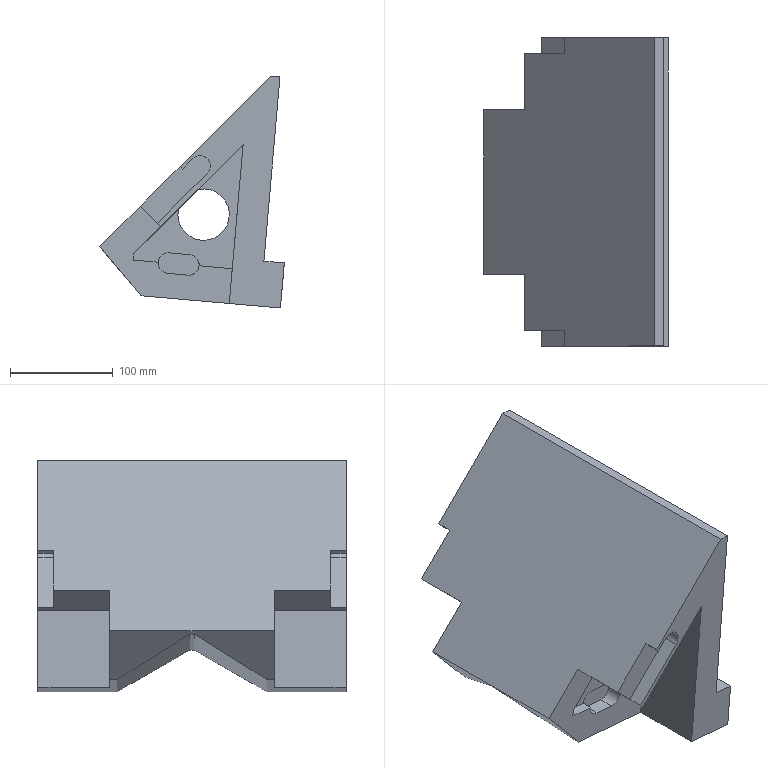Part | NX | features solid 2 | 1 solid | 52 faces | box 179.715 x 300 x 225.718 mm | volume 4183928 mm3 | plane 45 | cylinder 7 | commonest cylinder face diameters 20 x6 50 x1